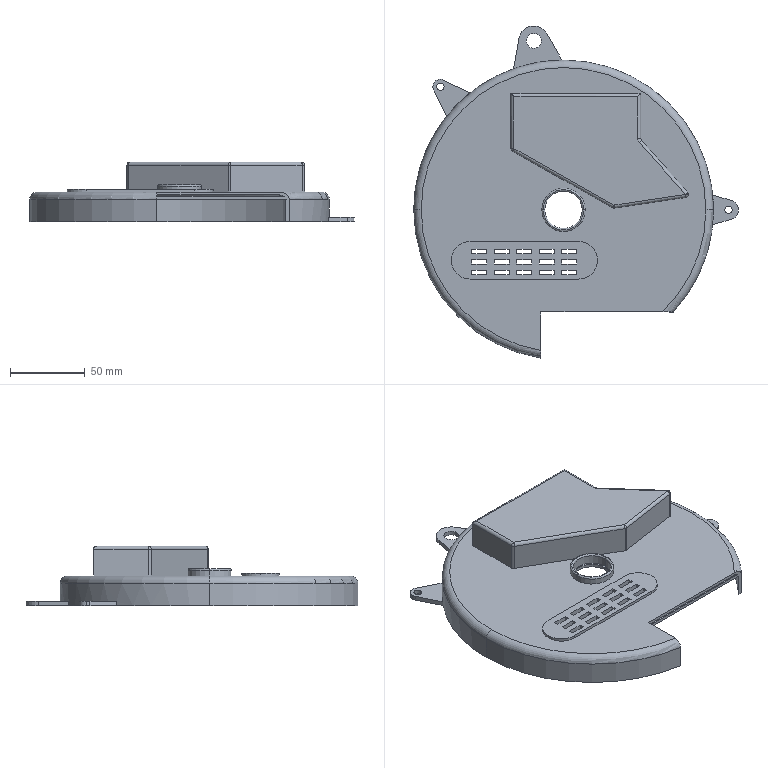Part | SolidWorks | features ICE 11, Fillet 3, Cut 1, Extrusion 1, Shell 1 | 1 solid | 212 faces | box 216.698 x 221.641 x 40 mm | volume 144146 mm3 | plane 158 | cylinder 39 | torus 11 | sphere 4 | commonest cylinder face diameters 4 x10 25 x7 10 x6 5 x4 196 x3 200 x3